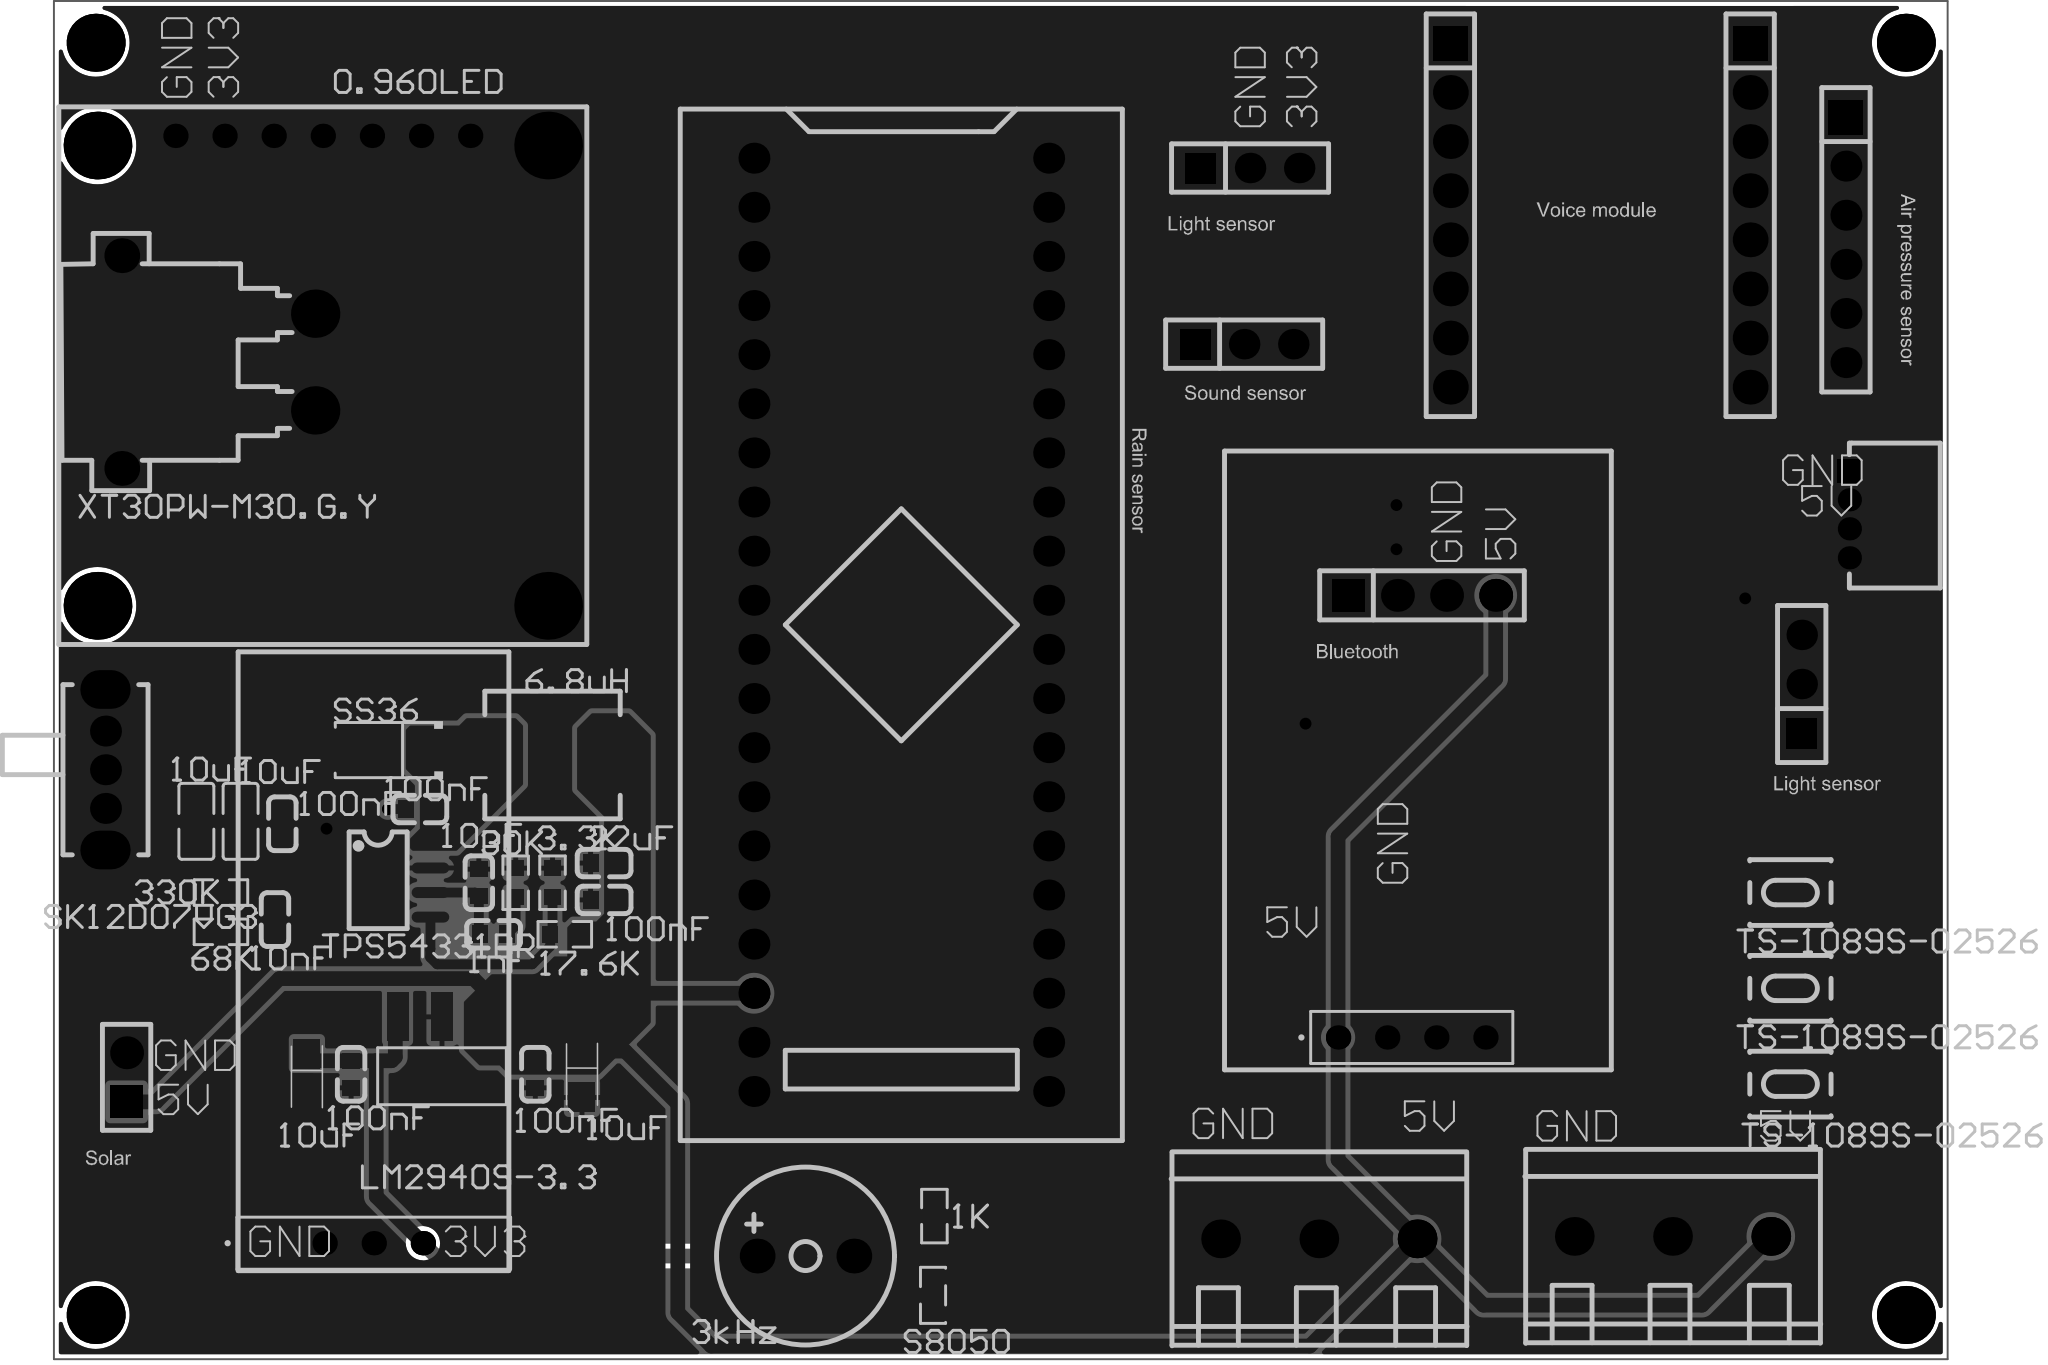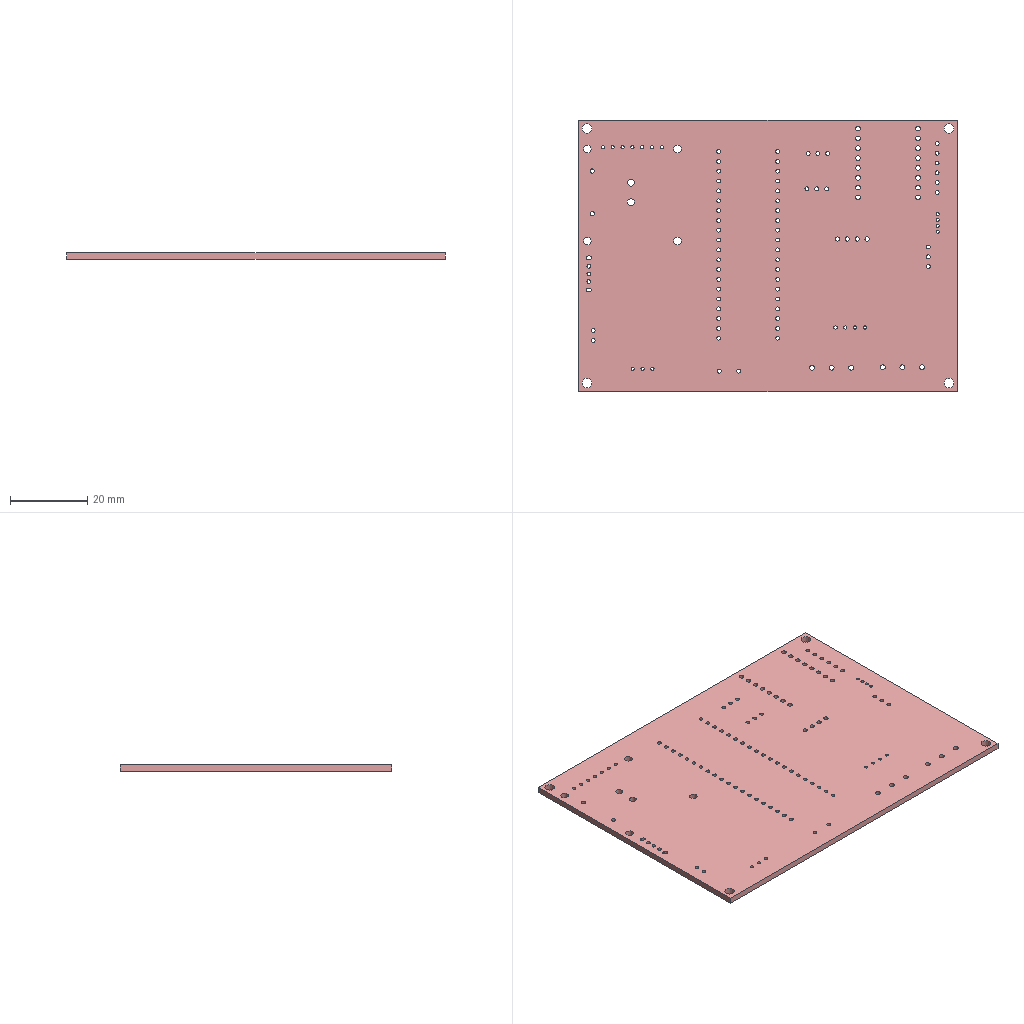Circuit board layout | Altium Designer | box 97.9 x 70.2 x 1.6 mm
Layer stack:
# Altium Designer layer stack of  (unit mm; dielectric type: 0 none, 1 core, 2 prepreg, 3 surface material)
index,name,kind,layer,copper_thickness_mm,dielectric_type,dielectric_thickness_mm,dielectric_material,dielectric_constant
0,Top Paste Mask Layer,other,,,,,,
1,Top Silkscreen Layer,other,,,,,,
2,Top Solder Mask Layer,dielectric,,,3,0.01,,3.3
3,Top Layer,copper,Top Layer,0.035,,,,
4,Dielectric1,dielectric,,,3,1.51,FR4,4.5
5,Bottom Layer,copper,Bottom Layer,0.035,,,,
6,Bottom Solder Mask Layer,dielectric,,,3,0.01,,3.3
7,Bottom Silkscreen Layer,other,,,,,,
8,Bottom Paste Mask Layer,other,,,,,,
# drill layer pairs: low layer,high layer
drill_pair,Top Layer,Bottom Layer
Part placement:
Designator,Comment,Layer,Footprint,Center-X(mm),Center-Y(mm),Rotation
BUZZER1,3kHz,TopLayer,BUZ-TH_BD9.0-P5.00-D0.6-FD,120.822,83.439,0
C11,10uF,TopLayer,CASE-A_3216,109.265,92.837,270
C12,10uF,TopLayer,CASE-A_3216,95.041,92.71,270
C13,100nF,TopLayer,C0603,97.327,92.837,90
C14,100nF,TopLayer,C0603,106.852,92.837,270
C25,100nF,TopLayer,C0603,93.771,105.791,270
C26,10nF,TopLayer,C0603,93.39,100.838,90
C27,10pF,TopLayer,C0603,103.931,102.743,270
C28,1nF,TopLayer,C0603,104.693,100.076,180
C29,100nF,TopLayer,C0603,100.883,106.553,0
C30,22uF,TopLayer,C0603,110.408,103.759,0
C31,100nF,TopLayer,C0603,110.408,101.854,0
C32,10uF,TopLayer,C0805,91.612,105.918,270
C33,10uF,TopLayer,C0805,89.326,105.918,270
CN1,XT30PW-M30.G.Y,TopLayer,CONN-TH_XT30PW-M,90.469,129.667,270
CN2,PM2.5 sensor,TopLayer,CONN-TH_4P-P1.50_HCTL_HC-ZH1.5-4AW,174.797,121.793,90
D2,SS36,TopLayer,SMA_L4.3-W2.6-LS5.2-RD,99.105,109.601,180
H1,Light sensor,TopLayer,HDR-TH_3P-P2.54-V-F,143.809,139.7,0
H2,Bluetooth,TopLayer,HDR-TH_4P-P2.54-V-F,152.699,117.602,0
L1,6.8uH,TopLayer,IND-SMD_L7.0-W6.6,107.741,109.347,0
P1,Wind speed sensor,TopLayer,CONN-TH_3P-P5.00_WJ500V-5.08-3P,147.365,84.328,0
P2,Wind direction sensor,TopLayer,CONN-TH_3P-P5.00_WJ500V-5.08-3P,165.653,84.455,0
Q1,S8050,TopLayer,SOT-23-3_L2.9-W1.3-P1.90-LS2.3-BR,127.426,81.407,0
R5,3.3K,TopLayer,R0603,107.741,102.743,270
R11,330K,TopLayer,R0603,90.596,102.235,180
R12,68K,TopLayer,R0603,90.596,100.203,0
R13,30K,TopLayer,R0603,105.836,102.743,270
R14,17.6K,TopLayer,R0603,108.376,100.076,0
R15,1K,TopLayer,R0603,127.487,85.505,270
SW1,SK12D07VG3,TopLayer,SW-TH_SK12D07VG3,84.627,108.585,270
SW2,TS-1089S-02526,TopLayer,SW-SMD_4P-L4.2-W3.3-P2.15-LS5.1,171.749,102.235,0
SW3,TS-1089S-02526,TopLayer,SW-SMD_4P-L4.2-W3.3-P2.15-LS5.1,171.749,97.282,0
SW4,TS-1089S-02526,TopLayer,SW-SMD_4P-L4.2-W3.3-P2.15-LS5.1,171.749,92.329,0
U1,LCKFB-DKX-STM32F103C8T6,TopLayer,CONN-TH_L53.3-W22.9_STM32F103C8T6-CARD,125.775,116.078,270
U6,LM2940S-3.3,TopLayer,SOT-223-3_L6.5-W3.4-P2.30-LS7.0-BR,102.026,92.837,90
U7,TPS54331DR,TopLayer,SOIC-8_L5.0-W4.0-P1.27-LS6.0-BL,98.724,102.87,270
U9,Rain sensor,TopLayer,MQ-2烟雾传感器模块,152.169,94.742,270
U10,DHT11 temperature and humidity sensor,TopLayer,DHT11温湿度模块,98.499,84.103,270
U11,0.96OLED,TopLayer,0.96寸OLED,95.864,129.212,0
H3,Air pressure sensor,TopLayer,HDR-TH_6P-P2.54-V-F,174.619,135.988,270
H4,Light sensor,TopLayer,HDR-TH_3P-P2.54-V-F,172.333,113.017,90
H5,Sound sensor,TopLayer,HDR-TH_3P-P2.54-V-F,143.503,130.592,0
H6,Voice module,TopLayer,HDR-TH_8P-P2.54-V-F-1,154.165,137.257,270
H7,,TopLayer,HDR-TH_8P-P2.54-V-F-1,169.666,137.257,270
H8,Solar,TopLayer,HDR-TH_2P-P2.54-V-F,85.719,92.68,90
Pad and via stacks:
# Altium Designer via and pad stacks of  (unit mm). Each distinct definition once, with the count of objects using it.
# via: kind,start_layer,end_layer,hole_mm,diameter_mm,mode(0 simple;1 top-mid-bottom;2 full stack),diameter_per_layer,count,example_net
# pad: kind,layer,hole_mm,hole_type(0 round;1 square;2 slot),plating,top_size,top_shape(1 round;2 rect;3 octagon;9 rounded rect),mid_size,bottom_size,mode,footprint,size_per_layer,count,example
pad,Multi-Layer,2.5,0,plated,3x3,1,3x3,3x3,0,,,4,1
pad,Multi-Layer,1,0,plated,1.8x1.8,1,1.8x1.8,1.8x1.8,0,BUZ-TH_BD9.0-P5.00-D0.6-FD,,2,BUZZER1.1
pad,Multi-Layer,1.8,0,plated,2.5x2.5,1,2.5x2.5,2.5x2.5,0,CONN-TH_XT30PW-M,,2,CN1.1
pad,Multi-Layer,1.1,0,plated,1.8x1.8,1,1.8x1.8,1.8x1.8,0,CONN-TH_XT30PW-M,,2,CN1.3
pad,Multi-Layer,0.8,0,plated,1.2x1.2,1,1.2x1.2,1.2x1.2,0,CONN-TH_4P-P1.50_HCTL_HC-ZH1.5-4AW,,3,CN2.1
pad,Multi-Layer,0.8,0,plated,1.2x1.2,2,1.2x1.2,1.2x1.2,0,CONN-TH_4P-P1.50_HCTL_HC-ZH1.5-4AW,,1,CN2.4
pad,Multi-Layer,1.02,0,plated,1.575x1.575,1,1.575x1.575,1.575x1.575,0,HDR-TH_3P-P2.54-V-F,,6,H1.3
pad,Multi-Layer,1.02,0,plated,1.575x1.575,2,1.575x1.575,1.575x1.575,0,HDR-TH_3P-P2.54-V-F,,3,H1.1
pad,Multi-Layer,1.1,0,plated,1.7x1.7,2,1.7x1.7,1.7x1.7,0,HDR-TH_4P-P2.54-V-F,,1,H2.1
pad,Multi-Layer,1.1,0,plated,1.7x1.7,1,1.7x1.7,1.7x1.7,0,HDR-TH_4P-P2.54-V-F,,3,H2.2
pad,Multi-Layer,1.3,0,plated,2x2,1,2x2,2x2,0,CONN-TH_3P-P5.00_WJ500V-5.08-3P,,6,P1.3
pad,Multi-Layer,1,0,plated,1.6x1.6,1,1.6x1.6,1.6x1.6,0,SW-TH_SK12D07VG3,,3,SW1.1
pad,Multi-Layer,1,2,plated,2.6x2,1,2.6x2,2.6x2,0,SW-TH_SK12D07VG3,,2,SW1.4
pad,Multi-Layer,1,0,plated,1.6x1.6,1,1.6x1.6,1.6x1.6,0,CONN-TH_L53.3-W22.9_STM32F103C8T6-CARD,,40,U1.1
pad,Multi-Layer,0.8401,0,plated,1.26x1.26,1,1.26x1.26,1.26x1.26,0,MQ-2\u00D1\u00CC\u00CE\u00ED\u00B4\u00AB\u00B8\u00D0\u00C6\u00F7\u00C4\u00A3\u00BF\u00E9,,4,U9.1
pad,Multi-Layer,0.8401,0,plated,1.26x1.26,1,1.26x1.26,1.26x1.26,0,DHT11\u00CE\u00C2\u00CA\u00AA\u00B6\u00C8\u00C4\u00A3\u00BF\u00E9,,3,U10.3
pad,Multi-Layer,2,0,plated,3.5x3.5,1,3.5x3.5,3.5x3.5,0,0.96\u00B4\u00E7OLED,,4,U11.8
pad,Multi-Layer,0.8401,0,plated,1.26x1.26,1,1.26x1.26,1.26x1.26,0,0.96\u00B4\u00E7OLED,,7,U11.1
pad,Multi-Layer,1.02,0,plated,1.6x1.6,1,1.6x1.6,1.6x1.6,0,HDR-TH_6P-P2.54-V-F,,5,H3.6
pad,Multi-Layer,1.02,0,plated,1.8x1.8,2,1.8x1.8,1.8x1.8,0,HDR-TH_6P-P2.54-V-F,,1,H3.1
pad,Multi-Layer,1.2,0,plated,1.8x1.8,2,1.8x1.8,1.8x1.8,0,HDR-TH_8P-P2.54-V-F-1,,2,H6.1
pad,Multi-Layer,1.2,0,plated,1.8x1.8,1,1.8x1.8,1.8x1.8,0,HDR-TH_8P-P2.54-V-F-1,,14,H6.2
pad,Multi-Layer,1,0,plated,1.7x1.7,2,1.7x1.7,1.7x1.7,0,HDR-TH_2P-P2.54-V-F,,1,H8.1
pad,Multi-Layer,1,0,plated,1.7x1.7,1,1.7x1.7,1.7x1.7,0,HDR-TH_2P-P2.54-V-F,,1,H8.2
pad,Top Layer,0,0,plated,1.5x1.359,2,1.5x1.359,1.5x1.359,0,CASE-A_3216,,4,C11.1
pad,Top Layer,0,0,plated,0.8x0.9,2,0.8x0.9,0.8x0.9,0,C0603,,18,C13.2
pad,Top Layer,0,0,plated,1.41x1.35,2,1.41x1.35,1.41x1.35,0,C0805,,4,C32.2
pad,Top Layer,0,0,plated,2x2,2,2x2,2x2,0,SMA_L4.3-W2.6-LS5.2-RD,,2,D2.2
pad,Top Layer,0,0,plated,2.4x3.2,2,2.4x3.2,2.4x3.2,0,IND-SMD_L7.0-W6.6,,2,L1.1
pad,Top Layer,0,0,plated,1.07x0.532,2,1.07x0.532,1.07x0.532,0,SOT-23-3_L2.9-W1.3-P1.90-LS2.3-BR,,3,Q1.3
pad,Top Layer,0,0,plated,0.8065x0.864,2,0.8065x0.864,0.8065x0.864,0,R0603,,12,R5.2
pad,Top Layer,0,0,plated,0.7x1.3,2,0.7x1.3,0.7x1.3,0,SW-SMD_4P-L4.2-W3.3-P2.15-LS5.1,,12,SW2.1
pad,Top Layer,0,0,plated,2.5x1.1,2,2.5x1.1,2.5x1.1,0,SOT-223-3_L6.5-W3.4-P2.30-LS7.0-BR,,3,U6.1
pad,Top Layer,0,0,plated,2.34x3.6,2,2.34x3.6,2.34x3.6,0,SOT-223-3_L6.5-W3.4-P2.30-LS7.0-BR,,1,U6.4
pad,Top Layer,0,0,plated,0.5684x1.95,1,0.5684x1.95,0.5684x1.95,0,SOIC-8_L5.0-W4.0-P1.27-LS6.0-BL,,8,U7.1
via,Top Layer,Bottom Layer,0.3048,0.61,0,,6,$1N2018
Copper pours:
name,layer,net,type(0 solid;1 hatched;2 none)
Top Layer-PGND,Top Layer,PGND,0
Top Layer-VBAT_KEY,Top Layer,VBAT_KEY,0
Top Layer-$1N2017,Top Layer,$1N2017,0
Top Layer-+5V,Top Layer,+5V,0
Bottom Layer-PGND,Bottom Layer,PGND,0
Design rules, without the lines most boards share:
# Altium Designer design rules of  (exported by Altium Designer, unit mm)
# columns: name | kind | enabled | priority | scope1 | scope2 | descriptor | typed fields (field=value)
Clearance | 0 | disabled | 4 | All | All | Clearance Constraint (Gap=5.984mil) (Disabled)(All),(All) | gap=0.152
BoardOutlineClearance | 63 | disabled | 4 | All | All | Board Clearance Constraint (Gap=0mil) (Disabled)(All) |
copperThickness1oz | 0 | enabled | 5 | All | All | Clearance Constraint (Gap=5.984mil) (All),(All) | gap=0.152
copperThickness1oz_1 | 63 | enabled | 5 | All | All | Board Clearance Constraint (Gap=0mil) (All) |
PolygonConnect | 20 | disabled | 1 | All | All | Polygon Connect Rule(Direct Connect )(Conductor Width=10mil) (Relief Angle=90 Angle) (Entries=4) (Air Gap Width=10mil) (Disabled)(All),(All) | connect_style(0=relief,1=direct,2=none)=1 relief_conductor_width=0.254 relief_entries=4
copperRegion | 20 | enabled | 2 | All | All | Polygon Connect Rule(Relief Connect )(Conductor Width=10mil) (Relief Angle=90 Angle) (Entries=4) (Air Gap Width=10mil) (All),(All) | connect_style(0=relief,1=direct,2=none)=0 relief_conductor_width=0.254 relief_entries=4
solderMaskExpansion | 13 | enabled | 2 | All | All | Solder Mask Expansion (Expansion =2.008mil) (All) | expansion=0.051